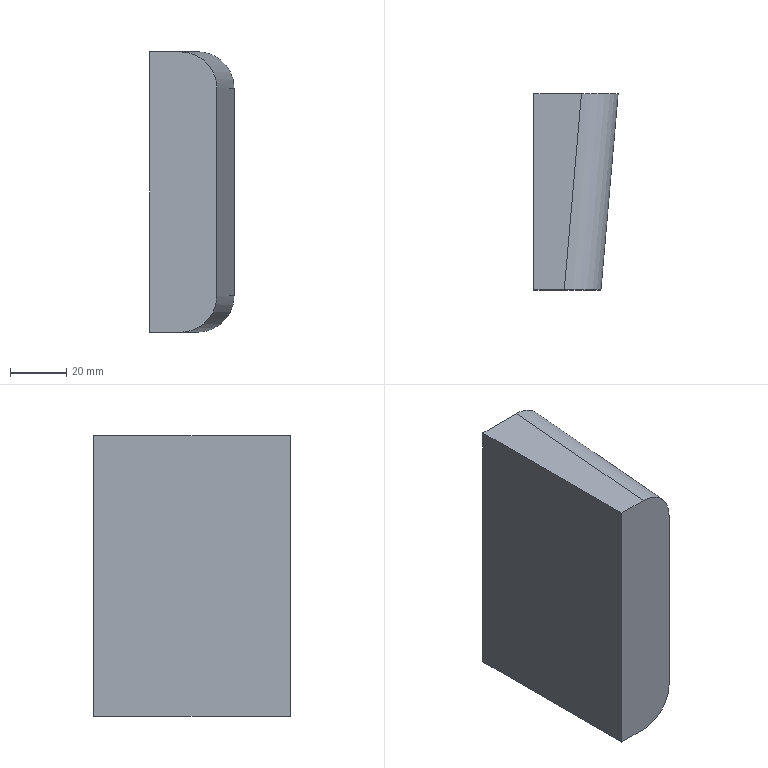Part | STEP file | 1 solid | 8 faces | box 30 x 70 x 100 mm | volume 183468 mm3 | plane 6 | cylinder 2 | commonest cylinder face diameters 26 x2
STEP:
#1=CARTESIAN_POINT('',(0.,0.,0.));
#2=DIRECTION('',(0.,0.,1.));
#3=DIRECTION('',(1.,0.,0.));
#4=AXIS2_PLACEMENT_3D('',#1,#2,#3);
#5=CARTESIAN_POINT('',(37.138,70.,-11.47));
#6=VERTEX_POINT('',#5);
#7=CARTESIAN_POINT('',(54.088,70.,-11.47));
#8=VERTEX_POINT('',#7);
#9=CARTESIAN_POINT('',(37.138,70.,-11.47));
#10=DIRECTION('',(1.,0.,0.));
#11=VECTOR('',#10,1.);
#12=LINE('',#9,#11);
#13=CARTESIAN_POINT('',(-72.862,70.,580.53));
#14=DIRECTION('',(0.,-1.,0.));
#15=DIRECTION('',(0.,0.,1.));
#16=AXIS2_PLACEMENT_3D('',#13,#14,#15);
#17=PLANE('',#16);
#18=CARTESIAN_POINT('',(-592.,-110.));
#19=DIRECTION('',(0.,-1.));
#20=VECTOR('',#19,1.);
#21=LINE('',#18,#20);
#22=(GEOMETRIC_REPRESENTATION_CONTEXT(2)PARAMETRIC_REPRESENTATION_CONTEXT()REPRESENTATION_CONTEXT('',''));
#23=DEFINITIONAL_REPRESENTATION('',(#21),#22);
#24=PCURVE('',#17,#23);
#25=CARTESIAN_POINT('',(37.138,150.,-11.47));
#26=DIRECTION('',(0.,0.,1.));
#27=DIRECTION('',(-1.,0.,0.));
#28=AXIS2_PLACEMENT_3D('',#25,#26,#27);
#29=PLANE('',#28);
#30=CARTESIAN_POINT('',(0.,80.));
#31=DIRECTION('',(-1.,0.));
#32=VECTOR('',#31,1.);
#33=LINE('',#30,#32);
#34=(GEOMETRIC_REPRESENTATION_CONTEXT(2)PARAMETRIC_REPRESENTATION_CONTEXT()REPRESENTATION_CONTEXT('',''));
#35=DEFINITIONAL_REPRESENTATION('',(#33),#34);
#36=PCURVE('',#29,#35);
#37=SURFACE_CURVE('',#12,(#24,#36),.PCURVE_S1.);
#38=EDGE_CURVE('',#6,#8,#37,.T.);
#39=ORIENTED_EDGE('',*,*,#38,.F.);
#40=CARTESIAN_POINT('',(37.138,70.,88.53));
#41=VERTEX_POINT('',#40);
#42=CARTESIAN_POINT('',(37.138,70.,88.53));
#43=DIRECTION('',(0.,0.,-1.));
#44=VECTOR('',#43,1.);
#45=LINE('',#42,#44);
#46=CARTESIAN_POINT('',(-492.,-110.));
#47=DIRECTION('',(-1.,0.));
#48=VECTOR('',#47,1.);
#49=LINE('',#46,#48);
#50=(GEOMETRIC_REPRESENTATION_CONTEXT(2)PARAMETRIC_REPRESENTATION_CONTEXT()REPRESENTATION_CONTEXT('',''));
#51=DEFINITIONAL_REPRESENTATION('',(#49),#50);
#52=PCURVE('',#17,#51);
#53=CARTESIAN_POINT('',(37.138,150.,88.53));
#54=DIRECTION('',(1.,0.,0.));
#55=DIRECTION('',(0.,0.,1.));
#56=AXIS2_PLACEMENT_3D('',#53,#54,#55);
#57=PLANE('',#56);
#58=CARTESIAN_POINT('',(0.,80.));
#59=DIRECTION('',(-1.,0.));
#60=VECTOR('',#59,1.);
#61=LINE('',#58,#60);
#62=(GEOMETRIC_REPRESENTATION_CONTEXT(2)PARAMETRIC_REPRESENTATION_CONTEXT()REPRESENTATION_CONTEXT('',''));
#63=DEFINITIONAL_REPRESENTATION('',(#61),#62);
#64=PCURVE('',#57,#63);
#65=SURFACE_CURVE('',#45,(#52,#64),.PCURVE_S1.);
#66=EDGE_CURVE('',#41,#6,#65,.T.);
#67=ORIENTED_EDGE('',*,*,#66,.F.);
#68=CARTESIAN_POINT('',(54.088,70.,88.53));
#69=VERTEX_POINT('',#68);
#70=CARTESIAN_POINT('',(57.138,70.,88.53));
#71=DIRECTION('',(-1.,0.,0.));
#72=VECTOR('',#71,1.);
#73=LINE('',#70,#72);
#74=CARTESIAN_POINT('',(-492.,-130.));
#75=DIRECTION('',(0.,1.));
#76=VECTOR('',#75,1.);
#77=LINE('',#74,#76);
#78=(GEOMETRIC_REPRESENTATION_CONTEXT(2)PARAMETRIC_REPRESENTATION_CONTEXT()REPRESENTATION_CONTEXT('',''));
#79=DEFINITIONAL_REPRESENTATION('',(#77),#78);
#80=PCURVE('',#17,#79);
#81=CARTESIAN_POINT('',(57.138,150.,88.53));
#82=DIRECTION('',(0.,0.,-1.));
#83=DIRECTION('',(1.,0.,0.));
#84=AXIS2_PLACEMENT_3D('',#81,#82,#83);
#85=PLANE('',#84);
#86=CARTESIAN_POINT('',(0.,80.));
#87=DIRECTION('',(-1.,0.));
#88=VECTOR('',#87,1.);
#89=LINE('',#86,#88);
#90=(GEOMETRIC_REPRESENTATION_CONTEXT(2)PARAMETRIC_REPRESENTATION_CONTEXT()REPRESENTATION_CONTEXT('',''));
#91=DEFINITIONAL_REPRESENTATION('',(#89),#90);
#92=PCURVE('',#85,#91);
#93=SURFACE_CURVE('',#73,(#80,#92),.PCURVE_S1.);
#94=EDGE_CURVE('',#69,#41,#93,.T.);
#95=ORIENTED_EDGE('',*,*,#94,.F.);
#96=CARTESIAN_POINT('',(67.138,70.,75.53));
#97=VERTEX_POINT('',#96);
#98=CARTESIAN_POINT('',(67.138,70.,75.53));
#99=CARTESIAN_POINT('',(67.138,70.,83.145));
#100=CARTESIAN_POINT('',(61.732,70.,88.53));
#101=CARTESIAN_POINT('',(54.088,70.,88.53));
#102=(BOUNDED_CURVE()B_SPLINE_CURVE(3,(#98,#99,#100,#101),.UNSPECIFIED.,.F.,.F.)B_SPLINE_CURVE_WITH_KNOTS((4,4),(3.142,4.712),.PIECEWISE_BEZIER_KNOTS.)CURVE()GEOMETRIC_REPRESENTATION_ITEM()RATIONAL_B_SPLINE_CURVE((1.,0.8047,0.8047,1.))REPRESENTATION_ITEM(''));
#103=CARTESIAN_POINT('',(-505.,-140.));
#104=CARTESIAN_POINT('',(-497.385,-140.));
#105=CARTESIAN_POINT('',(-492.,-134.595));
#106=CARTESIAN_POINT('',(-492.,-126.95));
#107=(BOUNDED_CURVE()B_SPLINE_CURVE(3,(#103,#104,#105,#106),.UNSPECIFIED.,.F.,.F.)B_SPLINE_CURVE_WITH_KNOTS((4,4),(3.142,4.712),.PIECEWISE_BEZIER_KNOTS.)CURVE()GEOMETRIC_REPRESENTATION_ITEM()RATIONAL_B_SPLINE_CURVE((1.,0.8047,0.8047,1.))REPRESENTATION_ITEM(''));
#108=(GEOMETRIC_REPRESENTATION_CONTEXT(2)PARAMETRIC_REPRESENTATION_CONTEXT()REPRESENTATION_CONTEXT('',''));
#109=DEFINITIONAL_REPRESENTATION('',(#107),#108);
#110=PCURVE('',#17,#109);
#111=CARTESIAN_POINT('',(61.057,149.657,75.53));
#112=DIRECTION('',(-0.08716,-0.9962,0.));
#113=DIRECTION('',(0.9962,-0.08716,0.));
#114=AXIS2_PLACEMENT_3D('',#111,#112,#113);
#115=CYLINDRICAL_SURFACE('',#114,13.);
#116=CARTESIAN_POINT('',(0.,78.824));
#117=CARTESIAN_POINT('',(0.02143,78.824));
#118=CARTESIAN_POINT('',(0.06485,78.826));
#119=CARTESIAN_POINT('',(0.1316,78.833));
#120=CARTESIAN_POINT('',(0.2,78.846));
#121=CARTESIAN_POINT('',(0.2697,78.864));
#122=CARTESIAN_POINT('',(0.3408,78.889));
#123=CARTESIAN_POINT('',(0.413,78.919));
#124=CARTESIAN_POINT('',(0.4863,78.955));
#125=CARTESIAN_POINT('',(0.5603,78.997));
#126=CARTESIAN_POINT('',(0.635,79.045));
#127=CARTESIAN_POINT('',(0.7101,79.098));
#128=CARTESIAN_POINT('',(0.7854,79.156));
#129=CARTESIAN_POINT('',(0.8607,79.219));
#130=CARTESIAN_POINT('',(0.9358,79.286));
#131=CARTESIAN_POINT('',(1.01,79.356));
#132=CARTESIAN_POINT('',(1.085,79.429));
#133=CARTESIAN_POINT('',(1.158,79.504));
#134=CARTESIAN_POINT('',(1.23,79.581));
#135=CARTESIAN_POINT('',(1.301,79.658));
#136=CARTESIAN_POINT('',(1.371,79.735));
#137=CARTESIAN_POINT('',(1.439,79.812));
#138=CARTESIAN_POINT('',(1.506,79.888));
#139=CARTESIAN_POINT('',(1.549,79.937));
#140=CARTESIAN_POINT('',(1.571,79.961));
#141=B_SPLINE_CURVE_WITH_KNOTS('',3,(#116,#117,#118,#119,#120,#121,#122,#123,#124,#125,#126,#127,#128,#129,#130,#131,#132,#133,#134,#135,#136,#137,#138,#139,#140),.UNSPECIFIED.,.F.,.F.,(4,1,1,1,1,1,1,1,1,1,1,1,1,1,1,1,1,1,1,1,1,1,4),(3.142,3.213,3.284,3.356,3.427,3.499,3.57,3.641,3.713,3.784,3.856,3.927,3.998,4.07,4.141,4.213,4.284,4.355,4.427,4.498,4.57,4.641,4.712),.QUASI_UNIFORM_KNOTS.);
#142=(GEOMETRIC_REPRESENTATION_CONTEXT(2)PARAMETRIC_REPRESENTATION_CONTEXT()REPRESENTATION_CONTEXT('',''));
#143=DEFINITIONAL_REPRESENTATION('',(#141),#142);
#144=PCURVE('',#115,#143);
#145=SURFACE_CURVE('',#102,(#110,#144),.PCURVE_S1.);
#146=EDGE_CURVE('',#97,#69,#145,.T.);
#147=ORIENTED_EDGE('',*,*,#146,.F.);
#148=CARTESIAN_POINT('',(67.138,70.,1.53));
#149=VERTEX_POINT('',#148);
#150=CARTESIAN_POINT('',(67.138,70.,38.53));
#151=DIRECTION('',(0.,0.,1.));
#152=VECTOR('',#151,1.);
#153=LINE('',#150,#152);
#154=CARTESIAN_POINT('',(-542.,-140.));
#155=DIRECTION('',(1.,0.));
#156=VECTOR('',#155,1.);
#157=LINE('',#154,#156);
#158=(GEOMETRIC_REPRESENTATION_CONTEXT(2)PARAMETRIC_REPRESENTATION_CONTEXT()REPRESENTATION_CONTEXT('',''));
#159=DEFINITIONAL_REPRESENTATION('',(#157),#158);
#160=PCURVE('',#17,#159);
#161=CARTESIAN_POINT('',(67.138,70.,38.53));
#162=DIRECTION('',(-0.9962,0.08716,0.));
#163=DIRECTION('',(-0.08716,-0.9962,0.));
#164=AXIS2_PLACEMENT_3D('',#161,#162,#163);
#165=PLANE('',#164);
#166=CARTESIAN_POINT('',(0.,0.));
#167=DIRECTION('',(0.,1.));
#168=VECTOR('',#167,1.);
#169=LINE('',#166,#168);
#170=(GEOMETRIC_REPRESENTATION_CONTEXT(2)PARAMETRIC_REPRESENTATION_CONTEXT()REPRESENTATION_CONTEXT('',''));
#171=DEFINITIONAL_REPRESENTATION('',(#169),#170);
#172=PCURVE('',#165,#171);
#173=SURFACE_CURVE('',#153,(#160,#172),.PCURVE_S1.);
#174=EDGE_CURVE('',#149,#97,#173,.T.);
#175=ORIENTED_EDGE('',*,*,#174,.F.);
#176=CARTESIAN_POINT('',(54.088,70.,-11.47));
#177=CARTESIAN_POINT('',(61.732,70.,-11.47));
#178=CARTESIAN_POINT('',(67.138,70.,-6.086));
#179=CARTESIAN_POINT('',(67.138,70.,1.53));
#180=(BOUNDED_CURVE()B_SPLINE_CURVE(3,(#176,#177,#178,#179),.UNSPECIFIED.,.F.,.F.)B_SPLINE_CURVE_WITH_KNOTS((4,4),(1.571,3.142),.PIECEWISE_BEZIER_KNOTS.)CURVE()GEOMETRIC_REPRESENTATION_ITEM()RATIONAL_B_SPLINE_CURVE((1.,0.8047,0.8047,1.))REPRESENTATION_ITEM(''));
#181=CARTESIAN_POINT('',(-592.,-126.95));
#182=CARTESIAN_POINT('',(-592.,-134.595));
#183=CARTESIAN_POINT('',(-586.615,-140.));
#184=CARTESIAN_POINT('',(-579.,-140.));
#185=(BOUNDED_CURVE()B_SPLINE_CURVE(3,(#181,#182,#183,#184),.UNSPECIFIED.,.F.,.F.)B_SPLINE_CURVE_WITH_KNOTS((4,4),(1.571,3.142),.PIECEWISE_BEZIER_KNOTS.)CURVE()GEOMETRIC_REPRESENTATION_ITEM()RATIONAL_B_SPLINE_CURVE((1.,0.8047,0.8047,1.))REPRESENTATION_ITEM(''));
#186=(GEOMETRIC_REPRESENTATION_CONTEXT(2)PARAMETRIC_REPRESENTATION_CONTEXT()REPRESENTATION_CONTEXT('',''));
#187=DEFINITIONAL_REPRESENTATION('',(#185),#186);
#188=PCURVE('',#17,#187);
#189=CARTESIAN_POINT('',(54.187,71.133,1.53));
#190=DIRECTION('',(-0.08716,-0.9962,0.));
#191=DIRECTION('',(0.9962,-0.08716,0.));
#192=AXIS2_PLACEMENT_3D('',#189,#190,#191);
#193=CYLINDRICAL_SURFACE('',#192,13.);
#194=CARTESIAN_POINT('',(4.712,1.137));
#195=CARTESIAN_POINT('',(4.734,1.113));
#196=CARTESIAN_POINT('',(4.777,1.064));
#197=CARTESIAN_POINT('',(4.844,0.988));
#198=CARTESIAN_POINT('',(4.912,0.9113));
#199=CARTESIAN_POINT('',(4.982,0.834));
#200=CARTESIAN_POINT('',(5.053,0.7569));
#201=CARTESIAN_POINT('',(5.125,0.6804));
#202=CARTESIAN_POINT('',(5.199,0.6054));
#203=CARTESIAN_POINT('',(5.273,0.5323));
#204=CARTESIAN_POINT('',(5.347,0.4621));
#205=CARTESIAN_POINT('',(5.422,0.3952));
#206=CARTESIAN_POINT('',(5.498,0.3324));
#207=CARTESIAN_POINT('',(5.573,0.2741));
#208=CARTESIAN_POINT('',(5.648,0.2208));
#209=CARTESIAN_POINT('',(5.723,0.173));
#210=CARTESIAN_POINT('',(5.797,0.1309));
#211=CARTESIAN_POINT('',(5.87,0.09472));
#212=CARTESIAN_POINT('',(5.942,0.06449));
#213=CARTESIAN_POINT('',(6.013,0.04021));
#214=CARTESIAN_POINT('',(6.083,0.02178));
#215=CARTESIAN_POINT('',(6.152,0.008981));
#216=CARTESIAN_POINT('',(6.218,0.001569));
#217=CARTESIAN_POINT('',(6.262,-0.000003694));
#218=CARTESIAN_POINT('',(6.283,0.));
#219=B_SPLINE_CURVE_WITH_KNOTS('',3,(#194,#195,#196,#197,#198,#199,#200,#201,#202,#203,#204,#205,#206,#207,#208,#209,#210,#211,#212,#213,#214,#215,#216,#217,#218),.UNSPECIFIED.,.F.,.F.,(4,1,1,1,1,1,1,1,1,1,1,1,1,1,1,1,1,1,1,1,1,1,4),(1.571,1.642,1.714,1.785,1.856,1.928,1.999,2.071,2.142,2.213,2.285,2.356,2.428,2.499,2.57,2.642,2.713,2.785,2.856,2.927,2.999,3.07,3.142),.QUASI_UNIFORM_KNOTS.);
#220=(GEOMETRIC_REPRESENTATION_CONTEXT(2)PARAMETRIC_REPRESENTATION_CONTEXT()REPRESENTATION_CONTEXT('',''));
#221=DEFINITIONAL_REPRESENTATION('',(#219),#220);
#222=PCURVE('',#193,#221);
#223=SURFACE_CURVE('',#180,(#188,#222),.PCURVE_S1.);
#224=EDGE_CURVE('',#8,#149,#223,.T.);
#225=ORIENTED_EDGE('',*,*,#224,.F.);
#226=EDGE_LOOP('',(#39,#67,#95,#147,#175,#225));
#227=FACE_BOUND('',#226,.T.);
#228=ADVANCED_FACE('',(#227),#17,.F.);
#229=ORIENTED_EDGE('',*,*,#94,.T.);
#230=CARTESIAN_POINT('',(37.138,0.,88.53));
#231=VERTEX_POINT('',#230);
#232=CARTESIAN_POINT('',(37.138,150.,88.53));
#233=DIRECTION('',(0.,-1.,0.));
#234=VECTOR('',#233,1.);
#235=LINE('',#232,#234);
#236=CARTESIAN_POINT('',(-20.,0.));
#237=DIRECTION('',(0.,1.));
#238=VECTOR('',#237,1.);
#239=LINE('',#236,#238);
#240=(GEOMETRIC_REPRESENTATION_CONTEXT(2)PARAMETRIC_REPRESENTATION_CONTEXT()REPRESENTATION_CONTEXT('',''));
#241=DEFINITIONAL_REPRESENTATION('',(#239),#240);
#242=PCURVE('',#85,#241);
#243=CARTESIAN_POINT('',(0.,0.));
#244=DIRECTION('',(0.,1.));
#245=VECTOR('',#244,1.);
#246=LINE('',#243,#245);
#247=(GEOMETRIC_REPRESENTATION_CONTEXT(2)PARAMETRIC_REPRESENTATION_CONTEXT()REPRESENTATION_CONTEXT('',''));
#248=DEFINITIONAL_REPRESENTATION('',(#246),#247);
#249=PCURVE('',#57,#248);
#250=SURFACE_CURVE('',#235,(#242,#249),.PCURVE_S1.);
#251=EDGE_CURVE('',#41,#231,#250,.T.);
#252=ORIENTED_EDGE('',*,*,#251,.T.);
#253=CARTESIAN_POINT('',(47.964,0.,88.53));
#254=VERTEX_POINT('',#253);
#255=CARTESIAN_POINT('',(57.138,0.,88.53));
#256=DIRECTION('',(-1.,0.,0.));
#257=VECTOR('',#256,1.);
#258=LINE('',#255,#257);
#259=CARTESIAN_POINT('',(0.,150.));
#260=DIRECTION('',(-1.,0.));
#261=VECTOR('',#260,1.);
#262=LINE('',#259,#261);
#263=(GEOMETRIC_REPRESENTATION_CONTEXT(2)PARAMETRIC_REPRESENTATION_CONTEXT()REPRESENTATION_CONTEXT('',''));
#264=DEFINITIONAL_REPRESENTATION('',(#262),#263);
#265=PCURVE('',#85,#264);
#266=CARTESIAN_POINT('',(52.138,0.,38.53));
#267=DIRECTION('',(0.,1.,0.));
#268=DIRECTION('',(0.,0.,-1.));
#269=AXIS2_PLACEMENT_3D('',#266,#267,#268);
#270=PLANE('',#269);
#271=CARTESIAN_POINT('',(-50.,-5.));
#272=DIRECTION('',(0.,1.));
#273=VECTOR('',#272,1.);
#274=LINE('',#271,#273);
#275=(GEOMETRIC_REPRESENTATION_CONTEXT(2)PARAMETRIC_REPRESENTATION_CONTEXT()REPRESENTATION_CONTEXT('',''));
#276=DEFINITIONAL_REPRESENTATION('',(#274),#275);
#277=PCURVE('',#270,#276);
#278=SURFACE_CURVE('',#258,(#265,#277),.PCURVE_S1.);
#279=EDGE_CURVE('',#254,#231,#278,.T.);
#280=ORIENTED_EDGE('',*,*,#279,.F.);
#281=CARTESIAN_POINT('',(61.057,149.657,88.53));
#282=DIRECTION('',(-0.08716,-0.9962,0.));
#283=VECTOR('',#282,1.);
#284=LINE('',#281,#283);
#285=CARTESIAN_POINT('',(3.919,0.3429));
#286=DIRECTION('',(-0.08716,0.9962));
#287=VECTOR('',#286,1.);
#288=LINE('',#285,#287);
#289=(GEOMETRIC_REPRESENTATION_CONTEXT(2)PARAMETRIC_REPRESENTATION_CONTEXT()REPRESENTATION_CONTEXT('',''));
#290=DEFINITIONAL_REPRESENTATION('',(#288),#289);
#291=PCURVE('',#85,#290);
#292=CARTESIAN_POINT('',(1.571,0.));
#293=DIRECTION('',(0.,1.));
#294=VECTOR('',#293,1.);
#295=LINE('',#292,#294);
#296=(GEOMETRIC_REPRESENTATION_CONTEXT(2)PARAMETRIC_REPRESENTATION_CONTEXT()REPRESENTATION_CONTEXT('',''));
#297=DEFINITIONAL_REPRESENTATION('',(#295),#296);
#298=PCURVE('',#115,#297);
#299=SURFACE_CURVE('',#284,(#291,#298),.PCURVE_S1.);
#300=EDGE_CURVE('',#69,#254,#299,.T.);
#301=ORIENTED_EDGE('',*,*,#300,.F.);
#302=EDGE_LOOP('',(#229,#252,#280,#301));
#303=FACE_BOUND('',#302,.T.);
#304=ADVANCED_FACE('',(#303),#85,.F.);
#305=ORIENTED_EDGE('',*,*,#174,.T.);
#306=CARTESIAN_POINT('',(61.013,0.,75.53));
#307=VERTEX_POINT('',#306);
#308=CARTESIAN_POINT('',(67.138,70.,75.53));
#309=DIRECTION('',(0.08716,0.9962,0.));
#310=VECTOR('',#309,1.);
#311=LINE('',#308,#310);
#312=CARTESIAN_POINT('',(0.,37.));
#313=DIRECTION('',(-1.,0.));
#314=VECTOR('',#313,1.);
#315=LINE('',#312,#314);
#316=(GEOMETRIC_REPRESENTATION_CONTEXT(2)PARAMETRIC_REPRESENTATION_CONTEXT()REPRESENTATION_CONTEXT('',''));
#317=DEFINITIONAL_REPRESENTATION('',(#315),#316);
#318=PCURVE('',#165,#317);
#319=CARTESIAN_POINT('',(0.,78.824));
#320=DIRECTION('',(0.,-1.));
#321=VECTOR('',#320,1.);
#322=LINE('',#319,#321);
#323=(GEOMETRIC_REPRESENTATION_CONTEXT(2)PARAMETRIC_REPRESENTATION_CONTEXT()REPRESENTATION_CONTEXT('',''));
#324=DEFINITIONAL_REPRESENTATION('',(#322),#323);
#325=PCURVE('',#115,#324);
#326=SURFACE_CURVE('',#311,(#318,#325),.PCURVE_S1.);
#327=EDGE_CURVE('',#307,#97,#326,.T.);
#328=ORIENTED_EDGE('',*,*,#327,.F.);
#329=CARTESIAN_POINT('',(61.013,0.,1.53));
#330=VERTEX_POINT('',#329);
#331=CARTESIAN_POINT('',(61.013,0.,38.53));
#332=DIRECTION('',(0.,0.,1.));
#333=VECTOR('',#332,1.);
#334=LINE('',#331,#333);
#335=CARTESIAN_POINT('',(70.267,0.));
#336=DIRECTION('',(0.,1.));
#337=VECTOR('',#336,1.);
#338=LINE('',#335,#337);
#339=(GEOMETRIC_REPRESENTATION_CONTEXT(2)PARAMETRIC_REPRESENTATION_CONTEXT()REPRESENTATION_CONTEXT('',''));
#340=DEFINITIONAL_REPRESENTATION('',(#338),#339);
#341=PCURVE('',#165,#340);
#342=CARTESIAN_POINT('',(0.,-8.876));
#343=DIRECTION('',(-1.,0.));
#344=VECTOR('',#343,1.);
#345=LINE('',#342,#344);
#346=(GEOMETRIC_REPRESENTATION_CONTEXT(2)PARAMETRIC_REPRESENTATION_CONTEXT()REPRESENTATION_CONTEXT('',''));
#347=DEFINITIONAL_REPRESENTATION('',(#345),#346);
#348=PCURVE('',#270,#347);
#349=SURFACE_CURVE('',#334,(#341,#348),.PCURVE_S1.);
#350=EDGE_CURVE('',#330,#307,#349,.T.);
#351=ORIENTED_EDGE('',*,*,#350,.F.);
#352=CARTESIAN_POINT('',(67.138,70.,1.53));
#353=DIRECTION('',(-0.08716,-0.9962,0.));
#354=VECTOR('',#353,1.);
#355=LINE('',#352,#354);
#356=CARTESIAN_POINT('',(0.,-37.));
#357=DIRECTION('',(1.,0.));
#358=VECTOR('',#357,1.);
#359=LINE('',#356,#358);
#360=(GEOMETRIC_REPRESENTATION_CONTEXT(2)PARAMETRIC_REPRESENTATION_CONTEXT()REPRESENTATION_CONTEXT('',''));
#361=DEFINITIONAL_REPRESENTATION('',(#359),#360);
#362=PCURVE('',#165,#361);
#363=CARTESIAN_POINT('',(6.283,0.));
#364=DIRECTION('',(0.,1.));
#365=VECTOR('',#364,1.);
#366=LINE('',#363,#365);
#367=(GEOMETRIC_REPRESENTATION_CONTEXT(2)PARAMETRIC_REPRESENTATION_CONTEXT()REPRESENTATION_CONTEXT('',''));
#368=DEFINITIONAL_REPRESENTATION('',(#366),#367);
#369=PCURVE('',#193,#368);
#370=SURFACE_CURVE('',#355,(#362,#369),.PCURVE_S1.);
#371=EDGE_CURVE('',#149,#330,#370,.T.);
#372=ORIENTED_EDGE('',*,*,#371,.F.);
#373=EDGE_LOOP('',(#305,#328,#351,#372));
#374=FACE_BOUND('',#373,.T.);
#375=ADVANCED_FACE('',(#374),#165,.F.);
#376=CARTESIAN_POINT('',(37.138,0.,-11.47));
#377=VERTEX_POINT('',#376);
#378=CARTESIAN_POINT('',(47.964,0.,-11.47));
#379=VERTEX_POINT('',#378);
#380=CARTESIAN_POINT('',(37.138,0.,-11.47));
#381=DIRECTION('',(1.,0.,0.));
#382=VECTOR('',#381,1.);
#383=LINE('',#380,#382);
#384=CARTESIAN_POINT('',(0.,150.));
#385=DIRECTION('',(-1.,0.));
#386=VECTOR('',#385,1.);
#387=LINE('',#384,#386);
#388=(GEOMETRIC_REPRESENTATION_CONTEXT(2)PARAMETRIC_REPRESENTATION_CONTEXT()REPRESENTATION_CONTEXT('',''));
#389=DEFINITIONAL_REPRESENTATION('',(#387),#388);
#390=PCURVE('',#29,#389);
#391=CARTESIAN_POINT('',(50.,15.));
#392=DIRECTION('',(0.,-1.));
#393=VECTOR('',#392,1.);
#394=LINE('',#391,#393);
#395=(GEOMETRIC_REPRESENTATION_CONTEXT(2)PARAMETRIC_REPRESENTATION_CONTEXT()REPRESENTATION_CONTEXT('',''));
#396=DEFINITIONAL_REPRESENTATION('',(#394),#395);
#397=PCURVE('',#270,#396);
#398=SURFACE_CURVE('',#383,(#390,#397),.PCURVE_S1.);
#399=EDGE_CURVE('',#377,#379,#398,.T.);
#400=ORIENTED_EDGE('',*,*,#399,.F.);
#401=CARTESIAN_POINT('',(37.138,150.,-11.47));
#402=DIRECTION('',(0.,-1.,0.));
#403=VECTOR('',#402,1.);
#404=LINE('',#401,#403);
#405=CARTESIAN_POINT('',(0.,0.));
#406=DIRECTION('',(0.,1.));
#407=VECTOR('',#406,1.);
#408=LINE('',#405,#407);
#409=(GEOMETRIC_REPRESENTATION_CONTEXT(2)PARAMETRIC_REPRESENTATION_CONTEXT()REPRESENTATION_CONTEXT('',''));
#410=DEFINITIONAL_REPRESENTATION('',(#408),#409);
#411=PCURVE('',#29,#410);
#412=CARTESIAN_POINT('',(-100.,0.));
#413=DIRECTION('',(0.,1.));
#414=VECTOR('',#413,1.);
#415=LINE('',#412,#414);
#416=(GEOMETRIC_REPRESENTATION_CONTEXT(2)PARAMETRIC_REPRESENTATION_CONTEXT()REPRESENTATION_CONTEXT('',''));
#417=DEFINITIONAL_REPRESENTATION('',(#415),#416);
#418=PCURVE('',#57,#417);
#419=SURFACE_CURVE('',#404,(#411,#418),.PCURVE_S1.);
#420=EDGE_CURVE('',#6,#377,#419,.T.);
#421=ORIENTED_EDGE('',*,*,#420,.F.);
#422=ORIENTED_EDGE('',*,*,#38,.T.);
#423=CARTESIAN_POINT('',(60.905,147.921,-11.47));
#424=DIRECTION('',(0.08716,0.9962,0.));
#425=VECTOR('',#424,1.);
#426=LINE('',#423,#425);
#427=CARTESIAN_POINT('',(-23.768,2.079));
#428=DIRECTION('',(-0.08716,-0.9962));
#429=VECTOR('',#428,1.);
#430=LINE('',#427,#429);
#431=(GEOMETRIC_REPRESENTATION_CONTEXT(2)PARAMETRIC_REPRESENTATION_CONTEXT()REPRESENTATION_CONTEXT('',''));
#432=DEFINITIONAL_REPRESENTATION('',(#430),#431);
#433=PCURVE('',#29,#432);
#434=CARTESIAN_POINT('',(4.712,-77.081));
#435=DIRECTION('',(0.,-1.));
#436=VECTOR('',#435,1.);
#437=LINE('',#434,#436);
#438=(GEOMETRIC_REPRESENTATION_CONTEXT(2)PARAMETRIC_REPRESENTATION_CONTEXT()REPRESENTATION_CONTEXT('',''));
#439=DEFINITIONAL_REPRESENTATION('',(#437),#438);
#440=PCURVE('',#193,#439);
#441=SURFACE_CURVE('',#426,(#433,#440),.PCURVE_S1.);
#442=EDGE_CURVE('',#379,#8,#441,.T.);
#443=ORIENTED_EDGE('',*,*,#442,.F.);
#444=EDGE_LOOP('',(#400,#421,#422,#443));
#445=FACE_BOUND('',#444,.T.);
#446=ADVANCED_FACE('',(#445),#29,.F.);
#447=ORIENTED_EDGE('',*,*,#251,.F.);
#448=ORIENTED_EDGE('',*,*,#66,.T.);
#449=ORIENTED_EDGE('',*,*,#420,.T.);
#450=CARTESIAN_POINT('',(37.138,0.,88.53));
#451=DIRECTION('',(0.,0.,-1.));
#452=VECTOR('',#451,1.);
#453=LINE('',#450,#452);
#454=CARTESIAN_POINT('',(0.,150.));
#455=DIRECTION('',(-1.,0.));
#456=VECTOR('',#455,1.);
#457=LINE('',#454,#456);
#458=(GEOMETRIC_REPRESENTATION_CONTEXT(2)PARAMETRIC_REPRESENTATION_CONTEXT()REPRESENTATION_CONTEXT('',''));
#459=DEFINITIONAL_REPRESENTATION('',(#457),#458);
#460=PCURVE('',#57,#459);
#461=CARTESIAN_POINT('',(-50.,15.));
#462=DIRECTION('',(1.,0.));
#463=VECTOR('',#462,1.);
#464=LINE('',#461,#463);
#465=(GEOMETRIC_REPRESENTATION_CONTEXT(2)PARAMETRIC_REPRESENTATION_CONTEXT()REPRESENTATION_CONTEXT('',''));
#466=DEFINITIONAL_REPRESENTATION('',(#464),#465);
#467=PCURVE('',#270,#466);
#468=SURFACE_CURVE('',#453,(#460,#467),.PCURVE_S1.);
#469=EDGE_CURVE('',#231,#377,#468,.T.);
#470=ORIENTED_EDGE('',*,*,#469,.F.);
#471=EDGE_LOOP('',(#447,#448,#449,#470));
#472=FACE_BOUND('',#471,.T.);
#473=ADVANCED_FACE('',(#472),#57,.F.);
#474=ORIENTED_EDGE('',*,*,#350,.T.);
#475=CARTESIAN_POINT('',(47.964,0.,88.53));
#476=CARTESIAN_POINT('',(55.608,0.,88.53));
#477=CARTESIAN_POINT('',(61.013,0.,83.145));
#478=CARTESIAN_POINT('',(61.013,0.,75.53));
#479=(BOUNDED_CURVE()B_SPLINE_CURVE(3,(#475,#476,#477,#478),.UNSPECIFIED.,.F.,.F.)B_SPLINE_CURVE_WITH_KNOTS((4,4),(1.571,3.142),.PIECEWISE_BEZIER_KNOTS.)CURVE()GEOMETRIC_REPRESENTATION_ITEM()RATIONAL_B_SPLINE_CURVE((1.,0.8047,0.8047,1.))REPRESENTATION_ITEM(''));
#480=CARTESIAN_POINT('',(-50.,4.174));
#481=CARTESIAN_POINT('',(-50.,-3.47));
#482=CARTESIAN_POINT('',(-44.615,-8.876));
#483=CARTESIAN_POINT('',(-37.,-8.876));
#484=(BOUNDED_CURVE()B_SPLINE_CURVE(3,(#480,#481,#482,#483),.UNSPECIFIED.,.F.,.F.)B_SPLINE_CURVE_WITH_KNOTS((4,4),(1.571,3.142),.PIECEWISE_BEZIER_KNOTS.)CURVE()GEOMETRIC_REPRESENTATION_ITEM()RATIONAL_B_SPLINE_CURVE((1.,0.8047,0.8047,1.))REPRESENTATION_ITEM(''));
#485=(GEOMETRIC_REPRESENTATION_CONTEXT(2)PARAMETRIC_REPRESENTATION_CONTEXT()REPRESENTATION_CONTEXT('',''));
#486=DEFINITIONAL_REPRESENTATION('',(#484),#485);
#487=PCURVE('',#270,#486);
#488=CARTESIAN_POINT('',(1.571,150.229));
#489=CARTESIAN_POINT('',(1.549,150.204));
#490=CARTESIAN_POINT('',(1.506,150.155));
#491=CARTESIAN_POINT('',(1.439,150.079));
#492=CARTESIAN_POINT('',(1.371,150.003));
#493=CARTESIAN_POINT('',(1.301,149.925));
#494=CARTESIAN_POINT('',(1.23,149.848));
#495=CARTESIAN_POINT('',(1.158,149.772));
#496=CARTESIAN_POINT('',(1.085,149.697));
#497=CARTESIAN_POINT('',(1.01,149.624));
#498=CARTESIAN_POINT('',(0.9358,149.553));
#499=CARTESIAN_POINT('',(0.8607,149.487));
#500=CARTESIAN_POINT('',(0.7854,149.424));
#501=CARTESIAN_POINT('',(0.7101,149.365));
#502=CARTESIAN_POINT('',(0.635,149.312));
#503=CARTESIAN_POINT('',(0.5603,149.264));
#504=CARTESIAN_POINT('',(0.4863,149.222));
#505=CARTESIAN_POINT('',(0.413,149.186));
#506=CARTESIAN_POINT('',(0.3408,149.156));
#507=CARTESIAN_POINT('',(0.2697,149.132));
#508=CARTESIAN_POINT('',(0.2,149.113));
#509=CARTESIAN_POINT('',(0.1316,149.1));
#510=CARTESIAN_POINT('',(0.06485,149.093));
#511=CARTESIAN_POINT('',(0.02143,149.091));
#512=CARTESIAN_POINT('',(0.,149.091));
#513=B_SPLINE_CURVE_WITH_KNOTS('',3,(#488,#489,#490,#491,#492,#493,#494,#495,#496,#497,#498,#499,#500,#501,#502,#503,#504,#505,#506,#507,#508,#509,#510,#511,#512),.UNSPECIFIED.,.F.,.F.,(4,1,1,1,1,1,1,1,1,1,1,1,1,1,1,1,1,1,1,1,1,1,4),(1.571,1.642,1.714,1.785,1.856,1.928,1.999,2.071,2.142,2.213,2.285,2.356,2.428,2.499,2.57,2.642,2.713,2.785,2.856,2.927,2.999,3.07,3.142),.QUASI_UNIFORM_KNOTS.);
#514=(GEOMETRIC_REPRESENTATION_CONTEXT(2)PARAMETRIC_REPRESENTATION_CONTEXT()REPRESENTATION_CONTEXT('',''));
#515=DEFINITIONAL_REPRESENTATION('',(#513),#514);
#516=PCURVE('',#115,#515);
#517=SURFACE_CURVE('',#479,(#487,#516),.PCURVE_S1.);
#518=EDGE_CURVE('',#254,#307,#517,.T.);
#519=ORIENTED_EDGE('',*,*,#518,.F.);
#520=ORIENTED_EDGE('',*,*,#279,.T.);
#521=ORIENTED_EDGE('',*,*,#469,.T.);
#522=ORIENTED_EDGE('',*,*,#399,.T.);
#523=CARTESIAN_POINT('',(61.013,0.,1.53));
#524=CARTESIAN_POINT('',(61.013,0.,-6.086));
#525=CARTESIAN_POINT('',(55.608,0.,-11.47));
#526=CARTESIAN_POINT('',(47.964,0.,-11.47));
#527=(BOUNDED_CURVE()B_SPLINE_CURVE(3,(#523,#524,#525,#526),.UNSPECIFIED.,.F.,.F.)B_SPLINE_CURVE_WITH_KNOTS((4,4),(3.142,4.712),.PIECEWISE_BEZIER_KNOTS.)CURVE()GEOMETRIC_REPRESENTATION_ITEM()RATIONAL_B_SPLINE_CURVE((1.,0.8047,0.8047,1.))REPRESENTATION_ITEM(''));
#528=CARTESIAN_POINT('',(37.,-8.876));
#529=CARTESIAN_POINT('',(44.615,-8.876));
#530=CARTESIAN_POINT('',(50.,-3.47));
#531=CARTESIAN_POINT('',(50.,4.174));
#532=(BOUNDED_CURVE()B_SPLINE_CURVE(3,(#528,#529,#530,#531),.UNSPECIFIED.,.F.,.F.)B_SPLINE_CURVE_WITH_KNOTS((4,4),(3.142,4.712),.PIECEWISE_BEZIER_KNOTS.)CURVE()GEOMETRIC_REPRESENTATION_ITEM()RATIONAL_B_SPLINE_CURVE((1.,0.8047,0.8047,1.))REPRESENTATION_ITEM(''));
#533=(GEOMETRIC_REPRESENTATION_CONTEXT(2)PARAMETRIC_REPRESENTATION_CONTEXT()REPRESENTATION_CONTEXT('',''));
#534=DEFINITIONAL_REPRESENTATION('',(#532),#533);
#535=PCURVE('',#270,#534);
#536=CARTESIAN_POINT('',(6.283,70.267));
#537=CARTESIAN_POINT('',(6.262,70.267));
#538=CARTESIAN_POINT('',(6.218,70.269));
#539=CARTESIAN_POINT('',(6.152,70.276));
#540=CARTESIAN_POINT('',(6.083,70.289));
#541=CARTESIAN_POINT('',(6.013,70.308));
#542=CARTESIAN_POINT('',(5.942,70.332));
#543=CARTESIAN_POINT('',(5.87,70.362));
#544=CARTESIAN_POINT('',(5.797,70.398));
#545=CARTESIAN_POINT('',(5.723,70.44));
#546=CARTESIAN_POINT('',(5.648,70.488));
#547=CARTESIAN_POINT('',(5.573,70.541));
#548=CARTESIAN_POINT('',(5.498,70.6));
#549=CARTESIAN_POINT('',(5.422,70.663));
#550=CARTESIAN_POINT('',(5.347,70.729));
#551=CARTESIAN_POINT('',(5.273,70.8));
#552=CARTESIAN_POINT('',(5.199,70.873));
#553=CARTESIAN_POINT('',(5.125,70.948));
#554=CARTESIAN_POINT('',(5.053,71.024));
#555=CARTESIAN_POINT('',(4.982,71.101));
#556=CARTESIAN_POINT('',(4.912,71.179));
#557=CARTESIAN_POINT('',(4.844,71.255));
#558=CARTESIAN_POINT('',(4.777,71.331));
#559=CARTESIAN_POINT('',(4.734,71.38));
#560=CARTESIAN_POINT('',(4.712,71.405));
#561=B_SPLINE_CURVE_WITH_KNOTS('',3,(#536,#537,#538,#539,#540,#541,#542,#543,#544,#545,#546,#547,#548,#549,#550,#551,#552,#553,#554,#555,#556,#557,#558,#559,#560),.UNSPECIFIED.,.F.,.F.,(4,1,1,1,1,1,1,1,1,1,1,1,1,1,1,1,1,1,1,1,1,1,4),(3.142,3.213,3.284,3.356,3.427,3.499,3.57,3.641,3.713,3.784,3.856,3.927,3.998,4.07,4.141,4.213,4.284,4.355,4.427,4.498,4.57,4.641,4.712),.QUASI_UNIFORM_KNOTS.);
#562=(GEOMETRIC_REPRESENTATION_CONTEXT(2)PARAMETRIC_REPRESENTATION_CONTEXT()REPRESENTATION_CONTEXT('',''));
#563=DEFINITIONAL_REPRESENTATION('',(#561),#562);
#564=PCURVE('',#193,#563);
#565=SURFACE_CURVE('',#527,(#535,#564),.PCURVE_S1.);
#566=EDGE_CURVE('',#330,#379,#565,.T.);
#567=ORIENTED_EDGE('',*,*,#566,.F.);
#568=EDGE_LOOP('',(#474,#519,#520,#521,#522,#567));
#569=FACE_BOUND('',#568,.T.);
#570=ADVANCED_FACE('',(#569),#270,.F.);
#571=ORIENTED_EDGE('',*,*,#224,.T.);
#572=ORIENTED_EDGE('',*,*,#371,.T.);
#573=ORIENTED_EDGE('',*,*,#566,.T.);
#574=ORIENTED_EDGE('',*,*,#442,.T.);
#575=EDGE_LOOP('',(#571,#572,#573,#574));
#576=FACE_BOUND('',#575,.T.);
#577=ADVANCED_FACE('',(#576),#193,.T.);
#578=ORIENTED_EDGE('',*,*,#146,.T.);
#579=ORIENTED_EDGE('',*,*,#300,.T.);
#580=ORIENTED_EDGE('',*,*,#518,.T.);
#581=ORIENTED_EDGE('',*,*,#327,.T.);
#582=EDGE_LOOP('',(#578,#579,#580,#581));
#583=FACE_BOUND('',#582,.T.);
#584=ADVANCED_FACE('',(#583),#115,.T.);
#585=CLOSED_SHELL('',(#228,#304,#375,#446,#473,#570,#577,#584));
#586=MANIFOLD_SOLID_BREP('',#585);
#587=(LENGTH_UNIT()NAMED_UNIT(*)SI_UNIT(.MILLI.,.METRE.));
#588=UNCERTAINTY_MEASURE_WITH_UNIT(LENGTH_MEASURE(0.0000001),#587,'','');
#589=(NAMED_UNIT(*)PLANE_ANGLE_UNIT()SI_UNIT($,.RADIAN.));
#590=(NAMED_UNIT(*)SI_UNIT($,.STERADIAN.)SOLID_ANGLE_UNIT());
#591=(GEOMETRIC_REPRESENTATION_CONTEXT(3)GLOBAL_UNCERTAINTY_ASSIGNED_CONTEXT((#588))GLOBAL_UNIT_ASSIGNED_CONTEXT((#587,#589,#590))REPRESENTATION_CONTEXT('',''));
#592=ADVANCED_BREP_SHAPE_REPRESENTATION('',(#4,#586),#591);